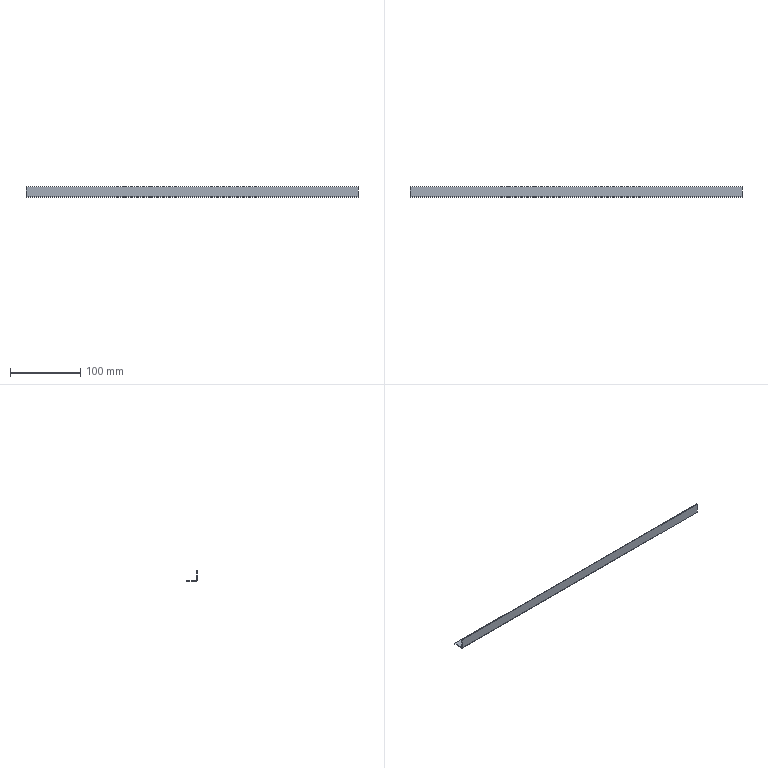Part | SolidWorks | features SplitBody 1 | 1 solid | 14 faces | box 471 x 15 x 15 mm | volume 13538 mm3 | plane 12 | cylinder 2 | commonest cylinder face diameters 0.2 x1 2.2 x1
STEP:
#1=CARTESIAN_POINT('',(498.,744.675,-297.9));
#2=VERTEX_POINT('',#1);
#3=CARTESIAN_POINT('',(498.,745.675,-297.9));
#4=VERTEX_POINT('',#3);
#5=CARTESIAN_POINT('',(498.,744.675,-297.9));
#6=DIRECTION('',(0.,1.,0.));
#7=VECTOR('',#6,1000.);
#8=LINE('',#5,#7);
#9=EDGE_CURVE('',#2,#4,#8,.T.);
#10=ORIENTED_EDGE('',*,*,#9,.F.);
#11=CARTESIAN_POINT('',(498.,745.775,-299.));
#12=VERTEX_POINT('',#11);
#13=CARTESIAN_POINT('',(498.,745.775,-297.9));
#14=DIRECTION('',(-1.,0.,0.));
#15=DIRECTION('',(0.,1.,0.));
#16=AXIS2_PLACEMENT_3D('',#13,#14,#15);
#17=CIRCLE('',#16,1.1);
#18=EDGE_CURVE('',#12,#2,#17,.T.);
#19=ORIENTED_EDGE('',*,*,#18,.F.);
#20=CARTESIAN_POINT('',(498.,745.775,-298.));
#21=VERTEX_POINT('',#20);
#22=CARTESIAN_POINT('',(498.,745.775,-298.));
#23=DIRECTION('',(0.,0.,-1.));
#24=VECTOR('',#23,1000.);
#25=LINE('',#22,#24);
#26=EDGE_CURVE('',#21,#12,#25,.T.);
#27=ORIENTED_EDGE('',*,*,#26,.F.);
#28=CARTESIAN_POINT('',(498.,745.775,-297.9));
#29=DIRECTION('',(-1.,0.,0.));
#30=DIRECTION('',(0.,0.,1.));
#31=AXIS2_PLACEMENT_3D('',#28,#29,#30);
#32=CIRCLE('',#31,0.1);
#33=EDGE_CURVE('',#21,#4,#32,.T.);
#34=ORIENTED_EDGE('',*,*,#33,.T.);
#35=EDGE_LOOP('',(#10,#19,#27,#34));
#36=FACE_OUTER_BOUND('',#35,.T.);
#37=CARTESIAN_POINT('',(498.,744.675,-297.9));
#38=DIRECTION('',(1.,0.,0.));
#39=DIRECTION('',(0.,1.,0.));
#40=AXIS2_PLACEMENT_3D('',#37,#38,#39);
#41=PLANE('',#40);
#42=ADVANCED_FACE('',(#36),#41,.T.);
#43=CARTESIAN_POINT('',(498.,744.675,-284.));
#44=VERTEX_POINT('',#43);
#45=CARTESIAN_POINT('',(498.,744.675,-299.));
#46=DIRECTION('',(0.,0.,1.));
#47=VECTOR('',#46,1000.);
#48=LINE('',#45,#47);
#49=EDGE_CURVE('',#2,#44,#48,.T.);
#50=ORIENTED_EDGE('',*,*,#49,.F.);
#51=ORIENTED_EDGE('',*,*,#9,.T.);
#52=CARTESIAN_POINT('',(498.,745.675,-284.));
#53=VERTEX_POINT('',#52);
#54=CARTESIAN_POINT('',(498.,745.675,-299.));
#55=DIRECTION('',(0.,0.,1.));
#56=VECTOR('',#55,1000.);
#57=LINE('',#54,#56);
#58=EDGE_CURVE('',#4,#53,#57,.T.);
#59=ORIENTED_EDGE('',*,*,#58,.T.);
#60=CARTESIAN_POINT('',(498.,745.675,-284.));
#61=DIRECTION('',(0.,-1.,0.));
#62=VECTOR('',#61,1000.);
#63=LINE('',#60,#62);
#64=EDGE_CURVE('',#53,#44,#63,.T.);
#65=ORIENTED_EDGE('',*,*,#64,.T.);
#66=EDGE_LOOP('',(#50,#51,#59,#65));
#67=FACE_OUTER_BOUND('',#66,.T.);
#68=CARTESIAN_POINT('',(498.,745.775,-298.));
#69=DIRECTION('',(1.,0.,0.));
#70=DIRECTION('',(0.,1.,0.));
#71=AXIS2_PLACEMENT_3D('',#68,#69,#70);
#72=PLANE('',#71);
#73=ADVANCED_FACE('',(#67),#72,.T.);
#74=CARTESIAN_POINT('',(27.,744.675,-284.));
#75=VERTEX_POINT('',#74);
#76=CARTESIAN_POINT('',(27.,744.675,-297.9));
#77=VERTEX_POINT('',#76);
#78=CARTESIAN_POINT('',(27.,744.675,-299.));
#79=DIRECTION('',(0.,0.,-1.));
#80=VECTOR('',#79,1000.);
#81=LINE('',#78,#80);
#82=EDGE_CURVE('',#75,#77,#81,.T.);
#83=ORIENTED_EDGE('',*,*,#82,.T.);
#84=CARTESIAN_POINT('',(5.787,744.675,-297.9));
#85=DIRECTION('',(1.,0.,0.));
#86=VECTOR('',#85,1000.);
#87=LINE('',#84,#86);
#88=EDGE_CURVE('',#77,#2,#87,.T.);
#89=ORIENTED_EDGE('',*,*,#88,.T.);
#90=ORIENTED_EDGE('',*,*,#49,.T.);
#91=CARTESIAN_POINT('',(5.787,744.675,-284.));
#92=DIRECTION('',(1.,0.,0.));
#93=VECTOR('',#92,1000.);
#94=LINE('',#91,#93);
#95=EDGE_CURVE('',#75,#44,#94,.T.);
#96=ORIENTED_EDGE('',*,*,#95,.F.);
#97=EDGE_LOOP('',(#83,#89,#90,#96));
#98=FACE_OUTER_BOUND('',#97,.T.);
#99=CARTESIAN_POINT('',(5.787,744.675,-299.));
#100=DIRECTION('',(0.,1.,0.));
#101=DIRECTION('',(-1.,0.,0.));
#102=AXIS2_PLACEMENT_3D('',#99,#100,#101);
#103=PLANE('',#102);
#104=ADVANCED_FACE('',(#98),#103,.F.);
#105=CARTESIAN_POINT('',(27.,745.675,-284.));
#106=VERTEX_POINT('',#105);
#107=CARTESIAN_POINT('',(5.787,745.675,-284.));
#108=DIRECTION('',(1.,0.,0.));
#109=VECTOR('',#108,1000.);
#110=LINE('',#107,#109);
#111=EDGE_CURVE('',#106,#53,#110,.T.);
#112=ORIENTED_EDGE('',*,*,#111,.F.);
#113=CARTESIAN_POINT('',(27.,744.675,-284.));
#114=DIRECTION('',(0.,1.,0.));
#115=VECTOR('',#114,1000.);
#116=LINE('',#113,#115);
#117=EDGE_CURVE('',#75,#106,#116,.T.);
#118=ORIENTED_EDGE('',*,*,#117,.F.);
#119=ORIENTED_EDGE('',*,*,#95,.T.);
#120=ORIENTED_EDGE('',*,*,#64,.F.);
#121=EDGE_LOOP('',(#112,#118,#119,#120));
#122=FACE_OUTER_BOUND('',#121,.T.);
#123=CARTESIAN_POINT('',(5.787,745.675,-284.));
#124=DIRECTION('',(0.,0.,1.));
#125=DIRECTION('',(1.,0.,0.));
#126=AXIS2_PLACEMENT_3D('',#123,#124,#125);
#127=PLANE('',#126);
#128=ADVANCED_FACE('',(#122),#127,.T.);
#129=CARTESIAN_POINT('',(27.,745.675,-297.9));
#130=VERTEX_POINT('',#129);
#131=CARTESIAN_POINT('',(5.787,745.675,-297.9));
#132=DIRECTION('',(1.,0.,0.));
#133=VECTOR('',#132,1000.);
#134=LINE('',#131,#133);
#135=EDGE_CURVE('',#130,#4,#134,.T.);
#136=ORIENTED_EDGE('',*,*,#135,.F.);
#137=CARTESIAN_POINT('',(27.,745.675,-299.));
#138=DIRECTION('',(0.,0.,-1.));
#139=VECTOR('',#138,1000.);
#140=LINE('',#137,#139);
#141=EDGE_CURVE('',#106,#130,#140,.T.);
#142=ORIENTED_EDGE('',*,*,#141,.F.);
#143=ORIENTED_EDGE('',*,*,#111,.T.);
#144=ORIENTED_EDGE('',*,*,#58,.F.);
#145=EDGE_LOOP('',(#136,#142,#143,#144));
#146=FACE_OUTER_BOUND('',#145,.T.);
#147=CARTESIAN_POINT('',(5.787,745.675,-299.));
#148=DIRECTION('',(0.,1.,0.));
#149=DIRECTION('',(-1.,0.,0.));
#150=AXIS2_PLACEMENT_3D('',#147,#148,#149);
#151=PLANE('',#150);
#152=ADVANCED_FACE('',(#146),#151,.T.);
#153=CARTESIAN_POINT('',(27.,745.775,-298.));
#154=VERTEX_POINT('',#153);
#155=CARTESIAN_POINT('',(5.787,745.775,-298.));
#156=DIRECTION('',(1.,0.,0.));
#157=VECTOR('',#156,1000.);
#158=LINE('',#155,#157);
#159=EDGE_CURVE('',#154,#21,#158,.T.);
#160=ORIENTED_EDGE('',*,*,#159,.F.);
#161=CARTESIAN_POINT('',(27.,745.775,-297.9));
#162=DIRECTION('',(1.,0.,0.));
#163=DIRECTION('',(0.,-1.,0.));
#164=AXIS2_PLACEMENT_3D('',#161,#162,#163);
#165=CIRCLE('',#164,0.1);
#166=EDGE_CURVE('',#130,#154,#165,.T.);
#167=ORIENTED_EDGE('',*,*,#166,.F.);
#168=ORIENTED_EDGE('',*,*,#135,.T.);
#169=ORIENTED_EDGE('',*,*,#33,.F.);
#170=EDGE_LOOP('',(#160,#167,#168,#169));
#171=FACE_OUTER_BOUND('',#170,.T.);
#172=CARTESIAN_POINT('',(5.787,745.775,-297.9));
#173=DIRECTION('',(1.,0.,0.));
#174=DIRECTION('',(0.,1.,0.));
#175=AXIS2_PLACEMENT_3D('',#172,#173,#174);
#176=CYLINDRICAL_SURFACE('',#175,0.1);
#177=ADVANCED_FACE('',(#171),#176,.F.);
#178=CARTESIAN_POINT('',(27.,759.675,-298.));
#179=VERTEX_POINT('',#178);
#180=CARTESIAN_POINT('',(498.,759.675,-298.));
#181=VERTEX_POINT('',#180);
#182=CARTESIAN_POINT('',(5.787,759.675,-298.));
#183=DIRECTION('',(1.,0.,0.));
#184=VECTOR('',#183,1000.);
#185=LINE('',#182,#184);
#186=EDGE_CURVE('',#179,#181,#185,.T.);
#187=ORIENTED_EDGE('',*,*,#186,.F.);
#188=CARTESIAN_POINT('',(27.,759.675,-298.));
#189=DIRECTION('',(0.,1.,0.));
#190=VECTOR('',#189,1000.);
#191=LINE('',#188,#190);
#192=EDGE_CURVE('',#154,#179,#191,.T.);
#193=ORIENTED_EDGE('',*,*,#192,.F.);
#194=ORIENTED_EDGE('',*,*,#159,.T.);
#195=CARTESIAN_POINT('',(498.,759.675,-298.));
#196=DIRECTION('',(0.,-1.,0.));
#197=VECTOR('',#196,1000.);
#198=LINE('',#195,#197);
#199=EDGE_CURVE('',#181,#21,#198,.T.);
#200=ORIENTED_EDGE('',*,*,#199,.F.);
#201=EDGE_LOOP('',(#187,#193,#194,#200));
#202=FACE_OUTER_BOUND('',#201,.T.);
#203=CARTESIAN_POINT('',(5.787,759.675,-298.));
#204=DIRECTION('',(0.,0.,1.));
#205=DIRECTION('',(1.,0.,0.));
#206=AXIS2_PLACEMENT_3D('',#203,#204,#205);
#207=PLANE('',#206);
#208=ADVANCED_FACE('',(#202),#207,.T.);
#209=CARTESIAN_POINT('',(27.,759.675,-299.));
#210=VERTEX_POINT('',#209);
#211=CARTESIAN_POINT('',(498.,759.675,-299.));
#212=VERTEX_POINT('',#211);
#213=CARTESIAN_POINT('',(5.787,759.675,-299.));
#214=DIRECTION('',(1.,0.,0.));
#215=VECTOR('',#214,1000.);
#216=LINE('',#213,#215);
#217=EDGE_CURVE('',#210,#212,#216,.T.);
#218=ORIENTED_EDGE('',*,*,#217,.F.);
#219=CARTESIAN_POINT('',(27.,759.675,-299.));
#220=DIRECTION('',(0.,0.,1.));
#221=VECTOR('',#220,1000.);
#222=LINE('',#219,#221);
#223=EDGE_CURVE('',#210,#179,#222,.T.);
#224=ORIENTED_EDGE('',*,*,#223,.T.);
#225=ORIENTED_EDGE('',*,*,#186,.T.);
#226=CARTESIAN_POINT('',(498.,759.675,-299.));
#227=DIRECTION('',(0.,0.,1.));
#228=VECTOR('',#227,1000.);
#229=LINE('',#226,#228);
#230=EDGE_CURVE('',#212,#181,#229,.T.);
#231=ORIENTED_EDGE('',*,*,#230,.F.);
#232=EDGE_LOOP('',(#218,#224,#225,#231));
#233=FACE_OUTER_BOUND('',#232,.T.);
#234=CARTESIAN_POINT('',(5.787,759.675,-299.));
#235=DIRECTION('',(0.,1.,0.));
#236=DIRECTION('',(-1.,0.,0.));
#237=AXIS2_PLACEMENT_3D('',#234,#235,#236);
#238=PLANE('',#237);
#239=ADVANCED_FACE('',(#233),#238,.T.);
#240=CARTESIAN_POINT('',(27.,745.775,-299.));
#241=VERTEX_POINT('',#240);
#242=CARTESIAN_POINT('',(27.,759.675,-299.));
#243=DIRECTION('',(0.,1.,0.));
#244=VECTOR('',#243,1000.);
#245=LINE('',#242,#244);
#246=EDGE_CURVE('',#241,#210,#245,.T.);
#247=ORIENTED_EDGE('',*,*,#246,.T.);
#248=ORIENTED_EDGE('',*,*,#217,.T.);
#249=CARTESIAN_POINT('',(498.,759.675,-299.));
#250=DIRECTION('',(0.,-1.,0.));
#251=VECTOR('',#250,1000.);
#252=LINE('',#249,#251);
#253=EDGE_CURVE('',#212,#12,#252,.T.);
#254=ORIENTED_EDGE('',*,*,#253,.T.);
#255=CARTESIAN_POINT('',(5.787,745.775,-299.));
#256=DIRECTION('',(1.,0.,0.));
#257=VECTOR('',#256,1000.);
#258=LINE('',#255,#257);
#259=EDGE_CURVE('',#241,#12,#258,.T.);
#260=ORIENTED_EDGE('',*,*,#259,.F.);
#261=EDGE_LOOP('',(#247,#248,#254,#260));
#262=FACE_OUTER_BOUND('',#261,.T.);
#263=CARTESIAN_POINT('',(5.787,759.675,-299.));
#264=DIRECTION('',(0.,0.,1.));
#265=DIRECTION('',(1.,0.,0.));
#266=AXIS2_PLACEMENT_3D('',#263,#264,#265);
#267=PLANE('',#266);
#268=ADVANCED_FACE('',(#262),#267,.F.);
#269=CARTESIAN_POINT('',(27.,745.775,-297.9));
#270=DIRECTION('',(1.,0.,0.));
#271=DIRECTION('',(0.,1.,0.));
#272=AXIS2_PLACEMENT_3D('',#269,#270,#271);
#273=CIRCLE('',#272,1.1);
#274=EDGE_CURVE('',#77,#241,#273,.T.);
#275=ORIENTED_EDGE('',*,*,#274,.T.);
#276=ORIENTED_EDGE('',*,*,#259,.T.);
#277=ORIENTED_EDGE('',*,*,#18,.T.);
#278=ORIENTED_EDGE('',*,*,#88,.F.);
#279=EDGE_LOOP('',(#275,#276,#277,#278));
#280=FACE_OUTER_BOUND('',#279,.T.);
#281=CARTESIAN_POINT('',(5.787,745.775,-297.9));
#282=DIRECTION('',(1.,0.,0.));
#283=DIRECTION('',(0.,1.,0.));
#284=AXIS2_PLACEMENT_3D('',#281,#282,#283);
#285=CYLINDRICAL_SURFACE('',#284,1.1);
#286=ADVANCED_FACE('',(#280),#285,.T.);
#287=ORIENTED_EDGE('',*,*,#199,.T.);
#288=ORIENTED_EDGE('',*,*,#26,.T.);
#289=ORIENTED_EDGE('',*,*,#253,.F.);
#290=ORIENTED_EDGE('',*,*,#230,.T.);
#291=EDGE_LOOP('',(#287,#288,#289,#290));
#292=FACE_OUTER_BOUND('',#291,.T.);
#293=CARTESIAN_POINT('',(498.,745.775,-297.9));
#294=DIRECTION('',(-1.,0.,0.));
#295=DIRECTION('',(0.,0.,1.));
#296=AXIS2_PLACEMENT_3D('',#293,#294,#295);
#297=PLANE('',#296);
#298=ADVANCED_FACE('',(#292),#297,.F.);
#299=CARTESIAN_POINT('',(27.,744.675,-297.9));
#300=DIRECTION('',(0.,1.,0.));
#301=VECTOR('',#300,1000.);
#302=LINE('',#299,#301);
#303=EDGE_CURVE('',#77,#130,#302,.T.);
#304=ORIENTED_EDGE('',*,*,#303,.F.);
#305=ORIENTED_EDGE('',*,*,#82,.F.);
#306=ORIENTED_EDGE('',*,*,#117,.T.);
#307=ORIENTED_EDGE('',*,*,#141,.T.);
#308=EDGE_LOOP('',(#304,#305,#306,#307));
#309=FACE_OUTER_BOUND('',#308,.T.);
#310=CARTESIAN_POINT('',(27.,744.675,-299.));
#311=DIRECTION('',(1.,0.,0.));
#312=DIRECTION('',(0.,0.,-1.));
#313=AXIS2_PLACEMENT_3D('',#310,#311,#312);
#314=PLANE('',#313);
#315=ADVANCED_FACE('',(#309),#314,.F.);
#316=ORIENTED_EDGE('',*,*,#223,.F.);
#317=ORIENTED_EDGE('',*,*,#246,.F.);
#318=CARTESIAN_POINT('',(27.,745.775,-299.));
#319=DIRECTION('',(0.,0.,1.));
#320=VECTOR('',#319,1000.);
#321=LINE('',#318,#320);
#322=EDGE_CURVE('',#241,#154,#321,.T.);
#323=ORIENTED_EDGE('',*,*,#322,.T.);
#324=ORIENTED_EDGE('',*,*,#192,.T.);
#325=EDGE_LOOP('',(#316,#317,#323,#324));
#326=FACE_OUTER_BOUND('',#325,.T.);
#327=CARTESIAN_POINT('',(27.,759.675,-299.));
#328=DIRECTION('',(1.,0.,0.));
#329=DIRECTION('',(0.,1.,0.));
#330=AXIS2_PLACEMENT_3D('',#327,#328,#329);
#331=PLANE('',#330);
#332=ADVANCED_FACE('',(#326),#331,.F.);
#333=ORIENTED_EDGE('',*,*,#166,.T.);
#334=ORIENTED_EDGE('',*,*,#322,.F.);
#335=ORIENTED_EDGE('',*,*,#274,.F.);
#336=ORIENTED_EDGE('',*,*,#303,.T.);
#337=EDGE_LOOP('',(#333,#334,#335,#336));
#338=FACE_OUTER_BOUND('',#337,.T.);
#339=CARTESIAN_POINT('',(27.,745.775,-297.9));
#340=DIRECTION('',(-1.,0.,0.));
#341=DIRECTION('',(0.,-1.,0.));
#342=AXIS2_PLACEMENT_3D('',#339,#340,#341);
#343=PLANE('',#342);
#344=ADVANCED_FACE('',(#338),#343,.T.);
#345=CLOSED_SHELL('',(#42,#73,#104,#128,#152,#177,#208,#239,#268,#286,#298,#315,#332,#344));
#346=MANIFOLD_SOLID_BREP('',#345);
#347=CARTESIAN_POINT('',(0.,0.,0.));
#348=DIRECTION('',(0.,0.,1.));
#349=DIRECTION('',(1.,0.,0.));
#350=AXIS2_PLACEMENT_3D('',#347,#348,#349);
#351=(LENGTH_UNIT()NAMED_UNIT(*)SI_UNIT(.MILLI.,.METRE.));
#352=UNCERTAINTY_MEASURE_WITH_UNIT(LENGTH_MEASURE(0.00001),#351,'','');
#353=(NAMED_UNIT(*)PLANE_ANGLE_UNIT()SI_UNIT($,.RADIAN.));
#354=(NAMED_UNIT(*)SI_UNIT($,.STERADIAN.)SOLID_ANGLE_UNIT());
#355=(GEOMETRIC_REPRESENTATION_CONTEXT(3)GLOBAL_UNCERTAINTY_ASSIGNED_CONTEXT((#352))GLOBAL_UNIT_ASSIGNED_CONTEXT((#351,#353,#354))REPRESENTATION_CONTEXT('',''));
#356=ADVANCED_BREP_SHAPE_REPRESENTATION('',(#346,#350),#355);